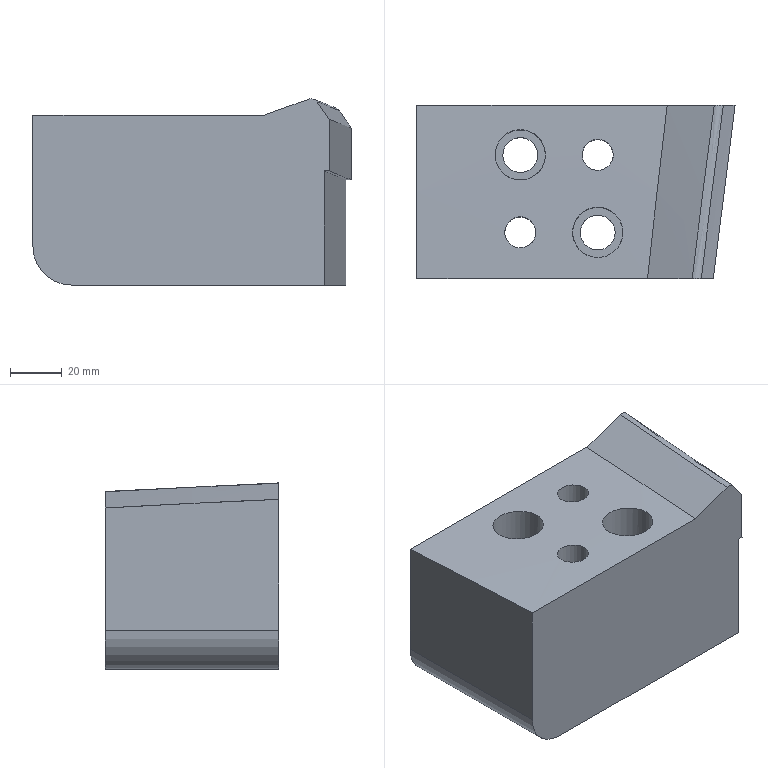Part | NX | features MAIN_BODY 2 | 1 solid | 20 faces | box 123.132 x 67 x 72.076 mm | volume 460289 mm3 | spline 7 | cylinder 7 | plane 6 | commonest cylinder face diameters 12 x2 13.5 x2 19.5 x2 30 x1
STEP:
#1=CARTESIAN_POINT('',(-841.75,399.358,-100.));
#2=VERTEX_POINT('',#1);
#3=CARTESIAN_POINT('',(-835.,399.358,-100.));
#4=DIRECTION('',(-0.000000341,-0.00000017,-1.));
#5=DIRECTION('',(-1.,0.,0.000000341));
#6=AXIS2_PLACEMENT_3D('',#3,#4,#5);
#7=CIRCLE('',#6,6.75);
#8=EDGE_CURVE('',#2,#2,#7,.F.);
#9=ORIENTED_EDGE('',*,*,#8,.T.);
#10=EDGE_LOOP('',(#9));
#11=FACE_BOUND('',#10,.T.);
#12=CARTESIAN_POINT('',(-841.,369.358,-100.));
#13=VERTEX_POINT('',#12);
#14=CARTESIAN_POINT('',(-835.,369.358,-100.));
#15=DIRECTION('',(-0.000000341,-0.00000017,-1.));
#16=DIRECTION('',(-1.,0.,0.000000341));
#17=AXIS2_PLACEMENT_3D('',#14,#15,#16);
#18=CIRCLE('',#17,6.);
#19=EDGE_CURVE('',#13,#13,#18,.F.);
#20=ORIENTED_EDGE('',*,*,#19,.T.);
#21=EDGE_LOOP('',(#20));
#22=FACE_BOUND('',#21,.T.);
#23=CARTESIAN_POINT('',(-811.75,369.358,-100.));
#24=VERTEX_POINT('',#23);
#25=CARTESIAN_POINT('',(-805.,369.358,-100.));
#26=DIRECTION('',(-0.000000341,-0.00000017,-1.));
#27=DIRECTION('',(-1.,0.,0.000000341));
#28=AXIS2_PLACEMENT_3D('',#25,#26,#27);
#29=CIRCLE('',#28,6.75);
#30=EDGE_CURVE('',#24,#24,#29,.F.);
#31=ORIENTED_EDGE('',*,*,#30,.T.);
#32=EDGE_LOOP('',(#31));
#33=FACE_BOUND('',#32,.T.);
#34=CARTESIAN_POINT('',(-811.,399.358,-100.));
#35=VERTEX_POINT('',#34);
#36=CARTESIAN_POINT('',(-805.,399.358,-100.));
#37=DIRECTION('',(-0.000000341,-0.00000017,-1.));
#38=DIRECTION('',(-1.,0.,0.000000341));
#39=AXIS2_PLACEMENT_3D('',#36,#37,#38);
#40=CIRCLE('',#39,6.);
#41=EDGE_CURVE('',#35,#35,#40,.F.);
#42=ORIENTED_EDGE('',*,*,#41,.T.);
#43=EDGE_LOOP('',(#42));
#44=FACE_BOUND('',#43,.T.);
#45=CARTESIAN_POINT('',(-860.,351.533,-100.));
#46=VERTEX_POINT('',#45);
#47=CARTESIAN_POINT('',(-762.297,351.533,-100.));
#48=VERTEX_POINT('',#47);
#49=CARTESIAN_POINT('',(-780.,351.533,-100.));
#50=DIRECTION('',(1.,0.000000011,-0.000000341));
#51=VECTOR('',#50,1000.);
#52=LINE('',#49,#51);
#53=EDGE_CURVE('',#46,#48,#52,.T.);
#54=ORIENTED_EDGE('',*,*,#53,.F.);
#55=CARTESIAN_POINT('',(-860.,418.533,-100.));
#56=VERTEX_POINT('',#55);
#57=CARTESIAN_POINT('',(-860.,1058.533,-100.));
#58=DIRECTION('',(-0.000000011,1.,-0.00000017));
#59=VECTOR('',#58,1000.);
#60=LINE('',#57,#59);
#61=EDGE_CURVE('',#46,#56,#60,.T.);
#62=ORIENTED_EDGE('',*,*,#61,.T.);
#63=CARTESIAN_POINT('',(-753.885,418.533,-100.));
#64=VERTEX_POINT('',#63);
#65=CARTESIAN_POINT('',(-780.,418.533,-100.));
#66=DIRECTION('',(1.,0.000000011,-0.000000341));
#67=VECTOR('',#66,1000.);
#68=LINE('',#65,#67);
#69=EDGE_CURVE('',#56,#64,#68,.T.);
#70=ORIENTED_EDGE('',*,*,#69,.T.);
#71=CARTESIAN_POINT('',(-753.885,418.533,-100.));
#72=CARTESIAN_POINT('',(-755.339,407.373,-100.));
#73=CARTESIAN_POINT('',(-758.303,385.059,-100.));
#74=CARTESIAN_POINT('',(-760.967,362.708,-100.));
#75=CARTESIAN_POINT('',(-762.297,351.533,-100.));
#76=B_SPLINE_CURVE_WITH_KNOTS('',3,(#71,#72,#73,#74,#75),.UNSPECIFIED.,.F.,.F.,(4,1,4),(0.2736,0.3074,0.3412),.UNSPECIFIED.);
#77=EDGE_CURVE('',#64,#48,#76,.T.);
#78=ORIENTED_EDGE('',*,*,#77,.T.);
#79=EDGE_LOOP('',(#54,#62,#70,#78));
#80=FACE_BOUND('',#79,.T.);
#81=CARTESIAN_POINT('',(-780.,1058.533,-100.));
#82=DIRECTION('',(-0.000000341,-0.00000017,-1.));
#83=DIRECTION('',(-0.000000011,1.,-0.00000017));
#84=AXIS2_PLACEMENT_3D('',#81,#82,#83);
#85=PLANE('',#84);
#86=ADVANCED_FACE('',(#11,#22,#33,#44,#80),#85,.T.);
#87=CARTESIAN_POINT('',(-751.868,418.533,-39.201));
#88=VERTEX_POINT('',#87);
#89=CARTESIAN_POINT('',(-756.435,418.533,-32.553));
#90=VERTEX_POINT('',#89);
#91=CARTESIAN_POINT('',(-751.868,418.533,-39.201));
#92=CARTESIAN_POINT('',(-753.39,418.533,-36.985));
#93=CARTESIAN_POINT('',(-754.912,418.533,-34.769));
#94=CARTESIAN_POINT('',(-756.435,418.533,-32.553));
#95=B_SPLINE_CURVE_WITH_KNOTS('',3,(#91,#92,#93,#94),.UNSPECIFIED.,.F.,.F.,(4,4),(0.,0.008065),.UNSPECIFIED.);
#96=EDGE_CURVE('',#88,#90,#95,.T.);
#97=ORIENTED_EDGE('',*,*,#96,.F.);
#98=CARTESIAN_POINT('',(-751.868,418.533,-59.201));
#99=VERTEX_POINT('',#98);
#100=CARTESIAN_POINT('',(-751.868,418.533,-39.201));
#101=CARTESIAN_POINT('',(-751.868,418.533,-45.868));
#102=CARTESIAN_POINT('',(-751.868,418.533,-52.535));
#103=CARTESIAN_POINT('',(-751.868,418.533,-59.201));
#104=B_SPLINE_CURVE_WITH_KNOTS('',3,(#100,#101,#102,#103),.UNSPECIFIED.,.F.,.F.,(4,4),(0.01625,0.03625),.UNSPECIFIED.);
#105=EDGE_CURVE('',#88,#99,#104,.T.);
#106=ORIENTED_EDGE('',*,*,#105,.T.);
#107=CARTESIAN_POINT('',(-753.885,418.533,-59.187));
#108=VERTEX_POINT('',#107);
#109=CARTESIAN_POINT('',(-753.885,418.533,-59.187));
#110=CARTESIAN_POINT('',(-753.213,418.533,-59.192));
#111=CARTESIAN_POINT('',(-752.541,418.533,-59.197));
#112=CARTESIAN_POINT('',(-751.868,418.533,-59.201));
#113=B_SPLINE_CURVE_WITH_KNOTS('',3,(#109,#110,#111,#112),.UNSPECIFIED.,.F.,.F.,(4,4),(0.,0.002017),.UNSPECIFIED.);
#114=EDGE_CURVE('',#108,#99,#113,.T.);
#115=ORIENTED_EDGE('',*,*,#114,.F.);
#116=CARTESIAN_POINT('',(-753.885,418.533,-59.187));
#117=CARTESIAN_POINT('',(-753.885,418.533,-72.791));
#118=CARTESIAN_POINT('',(-753.885,418.533,-86.396));
#119=CARTESIAN_POINT('',(-753.885,418.533,-100.));
#120=B_SPLINE_CURVE_WITH_KNOTS('',3,(#116,#117,#118,#119),.UNSPECIFIED.,.F.,.F.,(4,4),(-0.004527,0.03629),.UNSPECIFIED.);
#121=EDGE_CURVE('',#108,#64,#120,.T.);
#122=ORIENTED_EDGE('',*,*,#121,.T.);
#123=ORIENTED_EDGE('',*,*,#69,.F.);
#124=CARTESIAN_POINT('',(-875.,418.533,-85.));
#125=VERTEX_POINT('',#124);
#126=CARTESIAN_POINT('',(-860.,418.533,-85.));
#127=DIRECTION('',(-0.000000011,1.,-0.00000017));
#128=DIRECTION('',(0.,0.00000017,1.));
#129=AXIS2_PLACEMENT_3D('',#126,#127,#128);
#130=CIRCLE('',#129,15.);
#131=EDGE_CURVE('',#56,#125,#130,.T.);
#132=ORIENTED_EDGE('',*,*,#131,.T.);
#133=CARTESIAN_POINT('',(-875.,418.533,-37.652));
#134=VERTEX_POINT('',#133);
#135=CARTESIAN_POINT('',(-875.,418.533,-90.));
#136=DIRECTION('',(-0.000000341,-0.00000017,-1.));
#137=VECTOR('',#136,1000.);
#138=LINE('',#135,#137);
#139=EDGE_CURVE('',#125,#134,#138,.F.);
#140=ORIENTED_EDGE('',*,*,#139,.T.);
#141=CARTESIAN_POINT('',(-778.148,418.533,-37.652));
#142=VERTEX_POINT('',#141);
#143=CARTESIAN_POINT('',(-820.117,418.533,-37.652));
#144=DIRECTION('',(1.,0.000000011,-0.000000341));
#145=VECTOR('',#144,1000.);
#146=LINE('',#143,#145);
#147=EDGE_CURVE('',#134,#142,#146,.T.);
#148=ORIENTED_EDGE('',*,*,#147,.T.);
#149=CARTESIAN_POINT('',(-759.941,418.533,-31.393));
#150=VERTEX_POINT('',#149);
#151=CARTESIAN_POINT('',(-759.941,418.533,-31.393));
#152=CARTESIAN_POINT('',(-766.01,418.533,-33.479));
#153=CARTESIAN_POINT('',(-772.079,418.533,-35.565));
#154=CARTESIAN_POINT('',(-778.148,418.533,-37.652));
#155=B_SPLINE_CURVE_WITH_KNOTS('',3,(#151,#152,#153,#154),.UNSPECIFIED.,.F.,.F.,(4,4),(0.02556,0.04482),.UNSPECIFIED.);
#156=EDGE_CURVE('',#150,#142,#155,.T.);
#157=ORIENTED_EDGE('',*,*,#156,.F.);
#158=CARTESIAN_POINT('',(-756.435,418.533,-32.553));
#159=CARTESIAN_POINT('',(-757.19,418.533,-31.454));
#160=CARTESIAN_POINT('',(-758.679,418.533,-30.959));
#161=CARTESIAN_POINT('',(-759.941,418.533,-31.393));
#162=B_SPLINE_CURVE_WITH_KNOTS('',3,(#158,#159,#160,#161),.UNSPECIFIED.,.F.,.F.,(4,4),(0.,0.003944),.UNSPECIFIED.);
#163=EDGE_CURVE('',#90,#150,#162,.T.);
#164=ORIENTED_EDGE('',*,*,#163,.F.);
#165=EDGE_LOOP('',(#97,#106,#115,#122,#123,#132,#140,#148,#157,#164));
#166=FACE_BOUND('',#165,.T.);
#167=CARTESIAN_POINT('',(-840.,418.533,-90.));
#168=DIRECTION('',(-0.000000011,1.,-0.00000017));
#169=DIRECTION('',(0.000000341,0.00000017,1.));
#170=AXIS2_PLACEMENT_3D('',#167,#168,#169);
#171=PLANE('',#170);
#172=ADVANCED_FACE('',(#166),#171,.T.);
#173=CARTESIAN_POINT('',(-760.283,351.533,-35.819));
#174=VERTEX_POINT('',#173);
#175=CARTESIAN_POINT('',(-760.283,351.533,-55.819));
#176=VERTEX_POINT('',#175);
#177=CARTESIAN_POINT('',(-760.283,351.533,-35.819));
#178=CARTESIAN_POINT('',(-760.283,351.533,-42.486));
#179=CARTESIAN_POINT('',(-760.283,351.533,-49.152));
#180=CARTESIAN_POINT('',(-760.283,351.533,-55.819));
#181=B_SPLINE_CURVE_WITH_KNOTS('',3,(#177,#178,#179,#180),.UNSPECIFIED.,.F.,.F.,(4,4),(0.009058,0.02906),.UNSPECIFIED.);
#182=EDGE_CURVE('',#174,#176,#181,.T.);
#183=ORIENTED_EDGE('',*,*,#182,.T.);
#184=CARTESIAN_POINT('',(-751.868,418.533,-59.201));
#185=CARTESIAN_POINT('',(-753.322,407.375,-58.596));
#186=CARTESIAN_POINT('',(-756.286,385.067,-57.354));
#187=CARTESIAN_POINT('',(-758.953,362.711,-56.325));
#188=CARTESIAN_POINT('',(-760.283,351.533,-55.819));
#189=B_SPLINE_CURVE_WITH_KNOTS('',3,(#184,#185,#186,#187,#188),.UNSPECIFIED.,.F.,.F.,(4,1,4),(0.,0.03381,0.06761),.UNSPECIFIED.);
#190=EDGE_CURVE('',#99,#176,#189,.T.);
#191=ORIENTED_EDGE('',*,*,#190,.F.);
#192=ORIENTED_EDGE('',*,*,#105,.F.);
#193=CARTESIAN_POINT('',(-760.283,351.533,-35.819));
#194=CARTESIAN_POINT('',(-758.953,362.711,-36.325));
#195=CARTESIAN_POINT('',(-756.286,385.067,-37.354));
#196=CARTESIAN_POINT('',(-753.322,407.375,-38.596));
#197=CARTESIAN_POINT('',(-751.868,418.533,-39.201));
#198=B_SPLINE_CURVE_WITH_KNOTS('',3,(#193,#194,#195,#196,#197),.UNSPECIFIED.,.F.,.F.,(4,1,4),(0.,0.03381,0.06761),.UNSPECIFIED.);
#199=EDGE_CURVE('',#174,#88,#198,.T.);
#200=ORIENTED_EDGE('',*,*,#199,.F.);
#201=EDGE_LOOP('',(#183,#191,#192,#200));
#202=FACE_BOUND('',#201,.T.);
#203=CARTESIAN_POINT('',(-760.331,351.13,-55.941));
#204=CARTESIAN_POINT('',(-760.331,351.13,-35.657));
#205=CARTESIAN_POINT('',(-758.993,362.375,-56.467));
#206=CARTESIAN_POINT('',(-758.993,362.375,-36.183));
#207=CARTESIAN_POINT('',(-756.313,384.864,-57.522));
#208=CARTESIAN_POINT('',(-756.313,384.864,-37.238));
#209=CARTESIAN_POINT('',(-753.331,407.307,-58.731));
#210=CARTESIAN_POINT('',(-753.331,407.307,-38.447));
#211=CARTESIAN_POINT('',(-751.868,418.533,-59.322));
#212=CARTESIAN_POINT('',(-751.868,418.533,-39.037));
#213=B_SPLINE_SURFACE_WITH_KNOTS('',3,1,((#203,#204),(#205,#206),(#207,#208),(#209,#210),(#211,#212)),.SURF_OF_LINEAR_EXTRUSION.,.F.,.F.,.F.,(4,1,4),(2,2),(-0.3914,0.6746,1.741),(0.,1.),.UNSPECIFIED.);
#214=ADVANCED_FACE('',(#202),#213,.T.);
#215=ORIENTED_EDGE('',*,*,#139,.F.);
#216=CARTESIAN_POINT('',(-875.,351.533,-85.));
#217=VERTEX_POINT('',#216);
#218=CARTESIAN_POINT('',(-875.,739.25,-85.));
#219=DIRECTION('',(0.000000011,-1.,0.00000017));
#220=VECTOR('',#219,1000.);
#221=LINE('',#218,#220);
#222=EDGE_CURVE('',#125,#217,#221,.T.);
#223=ORIENTED_EDGE('',*,*,#222,.T.);
#224=CARTESIAN_POINT('',(-875.,351.533,-34.317));
#225=VERTEX_POINT('',#224);
#226=CARTESIAN_POINT('',(-875.,351.533,-90.));
#227=DIRECTION('',(-0.000000341,-0.00000017,-1.));
#228=VECTOR('',#227,1000.);
#229=LINE('',#226,#228);
#230=EDGE_CURVE('',#217,#225,#229,.F.);
#231=ORIENTED_EDGE('',*,*,#230,.T.);
#232=CARTESIAN_POINT('',(-875.,351.533,-34.317));
#233=CARTESIAN_POINT('',(-875.,373.874,-35.265));
#234=CARTESIAN_POINT('',(-875.,396.208,-36.367));
#235=CARTESIAN_POINT('',(-875.,418.533,-37.652));
#236=B_SPLINE_CURVE_WITH_KNOTS('',3,(#232,#233,#234,#235),.UNSPECIFIED.,.F.,.F.,(4,4),(0.277,0.3441),.UNSPECIFIED.);
#237=EDGE_CURVE('',#134,#225,#236,.F.);
#238=ORIENTED_EDGE('',*,*,#237,.F.);
#239=EDGE_LOOP('',(#215,#223,#231,#238));
#240=FACE_BOUND('',#239,.T.);
#241=CARTESIAN_POINT('',(-875.,739.25,-90.));
#242=DIRECTION('',(-1.,-0.000000011,0.000000341));
#243=DIRECTION('',(-0.000000341,-0.00000017,-1.));
#244=AXIS2_PLACEMENT_3D('',#241,#242,#243);
#245=PLANE('',#244);
#246=ADVANCED_FACE('',(#240),#245,.T.);
#247=CARTESIAN_POINT('',(-802.615,378.812,-35.56));
#248=VERTEX_POINT('',#247);
#249=CARTESIAN_POINT('',(-810.554,378.63,-35.551));
#250=CARTESIAN_POINT('',(-802.353,379.838,-35.61));
#251=CARTESIAN_POINT('',(-795.722,374.891,-35.371));
#252=CARTESIAN_POINT('',(-794.523,366.727,-34.987));
#253=CARTESIAN_POINT('',(-799.45,360.085,-34.688));
#254=CARTESIAN_POINT('',(-807.643,358.881,-34.635));
#255=CARTESIAN_POINT('',(-814.27,363.813,-34.854));
#256=CARTESIAN_POINT('',(-815.479,371.987,-35.232));
#257=CARTESIAN_POINT('',(-810.554,378.63,-35.551));
#258=CARTESIAN_POINT('',(-802.353,379.838,-35.61));
#259=CARTESIAN_POINT('',(-795.722,374.891,-35.371));
#260=B_SPLINE_CURVE_WITH_KNOTS('',3,(#249,#250,#251,#252,#253,#254,#255,#256,#257,#258,#259),.UNSPECIFIED.,.T.,.F.,(1,1,1,1,1,1,1,1,1,1,1,1,1,1,1),(-0.02287,-0.01525,-0.007624,0.,0.007624,0.01525,0.02287,0.0305,0.03812,0.04574,0.05337,0.06099,0.06862,0.07624,0.08386),.UNSPECIFIED.);
#261=EDGE_CURVE('',#248,#248,#260,.T.);
#262=ORIENTED_EDGE('',*,*,#261,.T.);
#263=EDGE_LOOP('',(#262));
#264=FACE_BOUND('',#263,.T.);
#265=CARTESIAN_POINT('',(-806.104,405.256,-36.91));
#266=VERTEX_POINT('',#265);
#267=CARTESIAN_POINT('',(-810.492,403.108,-36.793));
#268=CARTESIAN_POINT('',(-806.223,405.897,-36.944));
#269=CARTESIAN_POINT('',(-801.239,404.841,-36.887));
#270=CARTESIAN_POINT('',(-798.467,400.584,-36.658));
#271=CARTESIAN_POINT('',(-799.51,395.607,-36.398));
#272=CARTESIAN_POINT('',(-803.775,392.823,-36.256));
#273=CARTESIAN_POINT('',(-808.753,393.871,-36.309));
#274=CARTESIAN_POINT('',(-811.534,398.131,-36.529));
#275=CARTESIAN_POINT('',(-810.492,403.108,-36.793));
#276=CARTESIAN_POINT('',(-806.223,405.897,-36.944));
#277=CARTESIAN_POINT('',(-801.239,404.841,-36.887));
#278=B_SPLINE_CURVE_WITH_KNOTS('',3,(#267,#268,#269,#270,#271,#272,#273,#274,#275,#276,#277),.UNSPECIFIED.,.T.,.F.,(1,1,1,1,1,1,1,1,1,1,1,1,1,1,1),(-0.01408,-0.009385,-0.004692,0.,0.004692,0.009385,0.01408,0.01877,0.02346,0.02815,0.03285,0.03754,0.04223,0.04692,0.05162),.UNSPECIFIED.);
#279=EDGE_CURVE('',#266,#266,#278,.T.);
#280=ORIENTED_EDGE('',*,*,#279,.T.);
#281=EDGE_LOOP('',(#280));
#282=FACE_BOUND('',#281,.T.);
#283=CARTESIAN_POINT('',(-785.768,351.533,-34.317));
#284=VERTEX_POINT('',#283);
#285=CARTESIAN_POINT('',(-823.992,351.533,-34.317));
#286=DIRECTION('',(1.,0.000000011,-0.000000341));
#287=VECTOR('',#286,1000.);
#288=LINE('',#285,#287);
#289=EDGE_CURVE('',#225,#284,#288,.T.);
#290=ORIENTED_EDGE('',*,*,#289,.T.);
#291=CARTESIAN_POINT('',(-778.148,418.533,-37.652));
#292=CARTESIAN_POINT('',(-780.817,396.223,-36.368));
#293=CARTESIAN_POINT('',(-783.364,373.889,-35.266));
#294=CARTESIAN_POINT('',(-785.768,351.533,-34.317));
#295=B_SPLINE_CURVE_WITH_KNOTS('',3,(#291,#292,#293,#294),.UNSPECIFIED.,.F.,.F.,(4,4),(0.1671,0.2344),.UNSPECIFIED.);
#296=EDGE_CURVE('',#142,#284,#295,.T.);
#297=ORIENTED_EDGE('',*,*,#296,.F.);
#298=ORIENTED_EDGE('',*,*,#147,.F.);
#299=ORIENTED_EDGE('',*,*,#237,.T.);
#300=EDGE_LOOP('',(#290,#297,#298,#299));
#301=FACE_BOUND('',#300,.T.);
#302=CARTESIAN_POINT('',(-837.117,374.973,-35.376));
#303=VERTEX_POINT('',#302);
#304=CARTESIAN_POINT('',(-841.061,372.092,-35.239));
#305=CARTESIAN_POINT('',(-837.346,375.582,-35.405));
#306=CARTESIAN_POINT('',(-832.255,375.414,-35.397));
#307=CARTESIAN_POINT('',(-828.781,371.706,-35.22));
#308=CARTESIAN_POINT('',(-828.94,366.622,-34.983));
#309=CARTESIAN_POINT('',(-832.652,363.137,-34.825));
#310=CARTESIAN_POINT('',(-837.736,363.299,-34.832));
#311=CARTESIAN_POINT('',(-841.22,367.009,-35.001));
#312=CARTESIAN_POINT('',(-841.061,372.092,-35.239));
#313=CARTESIAN_POINT('',(-837.346,375.582,-35.405));
#314=CARTESIAN_POINT('',(-832.255,375.414,-35.397));
#315=B_SPLINE_CURVE_WITH_KNOTS('',3,(#304,#305,#306,#307,#308,#309,#310,#311,#312,#313,#314),.UNSPECIFIED.,.T.,.F.,(1,1,1,1,1,1,1,1,1,1,1,1,1,1,1),(-0.01408,-0.009384,-0.004692,0.,0.004692,0.009384,0.01408,0.01877,0.02346,0.02815,0.03284,0.03753,0.04223,0.04692,0.05161),.UNSPECIFIED.);
#316=EDGE_CURVE('',#303,#303,#315,.T.);
#317=ORIENTED_EDGE('',*,*,#316,.T.);
#318=EDGE_LOOP('',(#317));
#319=FACE_BOUND('',#318,.T.);
#320=CARTESIAN_POINT('',(-844.701,400.333,-36.646));
#321=VERTEX_POINT('',#320);
#322=CARTESIAN_POINT('',(-843.364,392.516,-36.238));
#323=CARTESIAN_POINT('',(-845.751,400.44,-36.648));
#324=CARTESIAN_POINT('',(-841.839,407.721,-37.043));
#325=CARTESIAN_POINT('',(-833.927,410.11,-37.176));
#326=CARTESIAN_POINT('',(-826.634,406.198,-36.959));
#327=CARTESIAN_POINT('',(-824.252,398.282,-36.535));
#328=CARTESIAN_POINT('',(-828.148,391.005,-36.162));
#329=CARTESIAN_POINT('',(-836.069,388.604,-36.043));
#330=CARTESIAN_POINT('',(-843.364,392.516,-36.238));
#331=CARTESIAN_POINT('',(-845.751,400.44,-36.648));
#332=CARTESIAN_POINT('',(-841.839,407.721,-37.043));
#333=B_SPLINE_CURVE_WITH_KNOTS('',3,(#322,#323,#324,#325,#326,#327,#328,#329,#330,#331,#332),.UNSPECIFIED.,.T.,.F.,(1,1,1,1,1,1,1,1,1,1,1,1,1,1,1),(-0.02288,-0.01525,-0.007625,0.,0.007625,0.01525,0.02288,0.0305,0.03813,0.04575,0.05338,0.061,0.06863,0.07625,0.08388),.UNSPECIFIED.);
#334=EDGE_CURVE('',#321,#321,#333,.T.);
#335=ORIENTED_EDGE('',*,*,#334,.T.);
#336=EDGE_LOOP('',(#335));
#337=FACE_BOUND('',#336,.T.);
#338=CARTESIAN_POINT('',(-875.586,418.533,-37.652));
#339=CARTESIAN_POINT('',(-776.779,418.533,-37.652));
#340=CARTESIAN_POINT('',(-877.041,407.36,-37.009));
#341=CARTESIAN_POINT('',(-778.234,407.36,-37.009));
#342=CARTESIAN_POINT('',(-880.005,385.084,-35.832));
#343=CARTESIAN_POINT('',(-781.198,385.084,-35.832));
#344=CARTESIAN_POINT('',(-882.657,362.711,-34.791));
#345=CARTESIAN_POINT('',(-783.85,362.711,-34.791));
#346=CARTESIAN_POINT('',(-883.99,351.533,-34.317));
#347=CARTESIAN_POINT('',(-785.183,351.533,-34.317));
#348=B_SPLINE_SURFACE_WITH_KNOTS('',3,1,((#338,#339),(#340,#341),(#342,#343),(#344,#345),(#346,#347)),.SURF_OF_LINEAR_EXTRUSION.,.F.,.F.,.F.,(4,1,4),(2,2),(-0.00601,0.4948,0.9956),(0.,1.),.UNSPECIFIED.);
#349=ADVANCED_FACE('',(#264,#282,#301,#319,#337),#348,.T.);
#350=CARTESIAN_POINT('',(-768.455,351.533,-28.093));
#351=VERTEX_POINT('',#350);
#352=CARTESIAN_POINT('',(-785.768,351.533,-34.317));
#353=CARTESIAN_POINT('',(-779.997,351.533,-32.242));
#354=CARTESIAN_POINT('',(-774.226,351.533,-30.167));
#355=CARTESIAN_POINT('',(-768.455,351.533,-28.093));
#356=B_SPLINE_CURVE_WITH_KNOTS('',3,(#352,#353,#354,#355),.UNSPECIFIED.,.F.,.F.,(4,4),(0.07252,0.09092),.UNSPECIFIED.);
#357=EDGE_CURVE('',#351,#284,#356,.F.);
#358=ORIENTED_EDGE('',*,*,#357,.T.);
#359=ORIENTED_EDGE('',*,*,#289,.F.);
#360=ORIENTED_EDGE('',*,*,#230,.F.);
#361=CARTESIAN_POINT('',(-860.,351.533,-85.));
#362=DIRECTION('',(-0.000000011,1.,-0.00000017));
#363=DIRECTION('',(0.,0.00000017,1.));
#364=AXIS2_PLACEMENT_3D('',#361,#362,#363);
#365=CIRCLE('',#364,15.);
#366=EDGE_CURVE('',#217,#46,#365,.F.);
#367=ORIENTED_EDGE('',*,*,#366,.T.);
#368=ORIENTED_EDGE('',*,*,#53,.T.);
#369=CARTESIAN_POINT('',(-762.297,351.533,-55.808));
#370=VERTEX_POINT('',#369);
#371=CARTESIAN_POINT('',(-762.297,351.533,-55.808));
#372=CARTESIAN_POINT('',(-762.297,351.533,-70.539));
#373=CARTESIAN_POINT('',(-762.297,351.533,-85.269));
#374=CARTESIAN_POINT('',(-762.297,351.533,-100.));
#375=B_SPLINE_CURVE_WITH_KNOTS('',3,(#371,#372,#373,#374),.UNSPECIFIED.,.F.,.F.,(4,4),(-0.01041,0.03379),.UNSPECIFIED.);
#376=EDGE_CURVE('',#370,#48,#375,.T.);
#377=ORIENTED_EDGE('',*,*,#376,.F.);
#378=CARTESIAN_POINT('',(-760.283,351.533,-55.819));
#379=CARTESIAN_POINT('',(-760.955,351.533,-55.816));
#380=CARTESIAN_POINT('',(-761.626,351.533,-55.812));
#381=CARTESIAN_POINT('',(-762.297,351.533,-55.808));
#382=B_SPLINE_CURVE_WITH_KNOTS('',3,(#378,#379,#380,#381),.UNSPECIFIED.,.F.,.F.,(4,4),(0.,0.002014),.UNSPECIFIED.);
#383=EDGE_CURVE('',#176,#370,#382,.T.);
#384=ORIENTED_EDGE('',*,*,#383,.F.);
#385=ORIENTED_EDGE('',*,*,#182,.F.);
#386=CARTESIAN_POINT('',(-764.943,351.533,-29.203));
#387=VERTEX_POINT('',#386);
#388=CARTESIAN_POINT('',(-764.943,351.533,-29.203));
#389=CARTESIAN_POINT('',(-763.39,351.533,-31.408));
#390=CARTESIAN_POINT('',(-761.836,351.533,-33.614));
#391=CARTESIAN_POINT('',(-760.283,351.533,-35.819));
#392=B_SPLINE_CURVE_WITH_KNOTS('',3,(#388,#389,#390,#391),.UNSPECIFIED.,.F.,.F.,(4,4),(0.007518,0.01561),.UNSPECIFIED.);
#393=EDGE_CURVE('',#387,#174,#392,.T.);
#394=ORIENTED_EDGE('',*,*,#393,.F.);
#395=CARTESIAN_POINT('',(-768.455,351.533,-28.093));
#396=CARTESIAN_POINT('',(-767.203,351.533,-27.643));
#397=CARTESIAN_POINT('',(-765.71,351.533,-28.115));
#398=CARTESIAN_POINT('',(-764.943,351.533,-29.203));
#399=B_SPLINE_CURVE_WITH_KNOTS('',3,(#395,#396,#397,#398),.UNSPECIFIED.,.F.,.F.,(4,4),(0.,0.003935),.UNSPECIFIED.);
#400=EDGE_CURVE('',#351,#387,#399,.T.);
#401=ORIENTED_EDGE('',*,*,#400,.F.);
#402=EDGE_LOOP('',(#358,#359,#360,#367,#368,#377,#384,#385,#394,#401));
#403=FACE_BOUND('',#402,.T.);
#404=CARTESIAN_POINT('',(-840.,351.533,-90.));
#405=DIRECTION('',(-0.000000011,1.,-0.00000017));
#406=DIRECTION('',(0.000000341,0.00000017,1.));
#407=AXIS2_PLACEMENT_3D('',#404,#405,#406);
#408=PLANE('',#407);
#409=ADVANCED_FACE('',(#403),#408,.F.);
#410=CARTESIAN_POINT('',(-844.75,399.358,-80.));
#411=VERTEX_POINT('',#410);
#412=CARTESIAN_POINT('',(-835.,399.358,-80.));
#413=DIRECTION('',(-0.000000341,-0.00000017,-1.));
#414=DIRECTION('',(-1.,0.,0.000000341));
#415=AXIS2_PLACEMENT_3D('',#412,#413,#414);
#416=CIRCLE('',#415,9.75);
#417=EDGE_CURVE('',#411,#411,#416,.F.);
#418=ORIENTED_EDGE('',*,*,#417,.F.);
#419=EDGE_LOOP('',(#418));
#420=FACE_BOUND('',#419,.T.);
#421=ORIENTED_EDGE('',*,*,#334,.F.);
#422=EDGE_LOOP('',(#421));
#423=FACE_BOUND('',#422,.T.);
#424=CARTESIAN_POINT('',(-835.,399.358,-70.));
#425=DIRECTION('',(0.000000341,0.00000017,1.));
#426=DIRECTION('',(0.000000011,-1.,0.00000017));
#427=AXIS2_PLACEMENT_3D('',#424,#425,#426);
#428=CYLINDRICAL_SURFACE('',#427,9.75);
#429=ADVANCED_FACE('',(#420,#423),#428,.F.);
#430=CARTESIAN_POINT('',(-841.75,399.358,-80.));
#431=VERTEX_POINT('',#430);
#432=CARTESIAN_POINT('',(-835.,399.358,-80.));
#433=DIRECTION('',(-0.000000341,-0.00000017,-1.));
#434=DIRECTION('',(-1.,0.,0.000000341));
#435=AXIS2_PLACEMENT_3D('',#432,#433,#434);
#436=CIRCLE('',#435,6.75);
#437=EDGE_CURVE('',#431,#431,#436,.F.);
#438=ORIENTED_EDGE('',*,*,#437,.T.);
#439=EDGE_LOOP('',(#438));
#440=FACE_BOUND('',#439,.T.);
#441=ORIENTED_EDGE('',*,*,#8,.F.);
#442=EDGE_LOOP('',(#441));
#443=FACE_BOUND('',#442,.T.);
#444=CARTESIAN_POINT('',(-835.,399.358,-90.));
#445=DIRECTION('',(0.000000341,0.00000017,1.));
#446=DIRECTION('',(0.000000011,-1.,0.00000017));
#447=AXIS2_PLACEMENT_3D('',#444,#445,#446);
#448=CYLINDRICAL_SURFACE('',#447,6.75);
#449=ADVANCED_FACE('',(#440,#443),#448,.F.);
#450=ORIENTED_EDGE('',*,*,#437,.F.);
#451=EDGE_LOOP('',(#450));
#452=FACE_BOUND('',#451,.T.);
#453=ORIENTED_EDGE('',*,*,#417,.T.);
#454=EDGE_LOOP('',(#453));
#455=FACE_BOUND('',#454,.T.);
#456=CARTESIAN_POINT('',(-835.,399.358,-80.));
#457=DIRECTION('',(-0.000000341,-0.00000017,-1.));
#458=DIRECTION('',(-0.000000011,1.,-0.00000017));
#459=AXIS2_PLACEMENT_3D('',#456,#457,#458);
#460=PLANE('',#459);
#461=ADVANCED_FACE('',(#452,#455),#460,.F.);
#462=ORIENTED_EDGE('',*,*,#19,.F.);
#463=EDGE_LOOP('',(#462));
#464=FACE_BOUND('',#463,.T.);
#465=ORIENTED_EDGE('',*,*,#316,.F.);
#466=EDGE_LOOP('',(#465));
#467=FACE_BOUND('',#466,.T.);
#468=CARTESIAN_POINT('',(-835.,369.358,-90.));
#469=DIRECTION('',(0.000000341,0.00000017,1.));
#470=DIRECTION('',(0.000000011,-1.,0.00000017));
#471=AXIS2_PLACEMENT_3D('',#468,#469,#470);
#472=CYLINDRICAL_SURFACE('',#471,6.);
#473=ADVANCED_FACE('',(#464,#467),#472,.F.);
#474=CARTESIAN_POINT('',(-814.75,369.358,-80.));
#475=VERTEX_POINT('',#474);
#476=CARTESIAN_POINT('',(-805.,369.358,-80.));
#477=DIRECTION('',(-0.000000341,-0.00000017,-1.));
#478=DIRECTION('',(-1.,0.,0.000000341));
#479=AXIS2_PLACEMENT_3D('',#476,#477,#478);
#480=CIRCLE('',#479,9.75);
#481=EDGE_CURVE('',#475,#475,#480,.F.);
#482=ORIENTED_EDGE('',*,*,#481,.F.);
#483=EDGE_LOOP('',(#482));
#484=FACE_BOUND('',#483,.T.);
#485=ORIENTED_EDGE('',*,*,#261,.F.);
#486=EDGE_LOOP('',(#485));
#487=FACE_BOUND('',#486,.T.);
#488=CARTESIAN_POINT('',(-805.,369.358,-70.));
#489=DIRECTION('',(0.000000341,0.00000017,1.));
#490=DIRECTION('',(0.000000011,-1.,0.00000017));
#491=AXIS2_PLACEMENT_3D('',#488,#489,#490);
#492=CYLINDRICAL_SURFACE('',#491,9.75);
#493=ADVANCED_FACE('',(#484,#487),#492,.F.);
#494=CARTESIAN_POINT('',(-811.75,369.358,-80.));
#495=VERTEX_POINT('',#494);
#496=CARTESIAN_POINT('',(-805.,369.358,-80.));
#497=DIRECTION('',(-0.000000341,-0.00000017,-1.));
#498=DIRECTION('',(-1.,0.,0.000000341));
#499=AXIS2_PLACEMENT_3D('',#496,#497,#498);
#500=CIRCLE('',#499,6.75);
#501=EDGE_CURVE('',#495,#495,#500,.F.);
#502=ORIENTED_EDGE('',*,*,#501,.T.);
#503=EDGE_LOOP('',(#502));
#504=FACE_BOUND('',#503,.T.);
#505=ORIENTED_EDGE('',*,*,#30,.F.);
#506=EDGE_LOOP('',(#505));
#507=FACE_BOUND('',#506,.T.);
#508=CARTESIAN_POINT('',(-805.,369.358,-90.));
#509=DIRECTION('',(0.000000341,0.00000017,1.));
#510=DIRECTION('',(0.000000011,-1.,0.00000017));
#511=AXIS2_PLACEMENT_3D('',#508,#509,#510);
#512=CYLINDRICAL_SURFACE('',#511,6.75);
#513=ADVANCED_FACE('',(#504,#507),#512,.F.);
#514=ORIENTED_EDGE('',*,*,#501,.F.);
#515=EDGE_LOOP('',(#514));
#516=FACE_BOUND('',#515,.T.);
#517=ORIENTED_EDGE('',*,*,#481,.T.);
#518=EDGE_LOOP('',(#517));
#519=FACE_BOUND('',#518,.T.);
#520=CARTESIAN_POINT('',(-805.,369.358,-80.));
#521=DIRECTION('',(-0.000000341,-0.00000017,-1.));
#522=DIRECTION('',(-0.000000011,1.,-0.00000017));
#523=AXIS2_PLACEMENT_3D('',#520,#521,#522);
#524=PLANE('',#523);
#525=ADVANCED_FACE('',(#516,#519),#524,.F.);
#526=ORIENTED_EDGE('',*,*,#41,.F.);
#527=EDGE_LOOP('',(#526));
#528=FACE_BOUND('',#527,.T.);
#529=ORIENTED_EDGE('',*,*,#279,.F.);
#530=EDGE_LOOP('',(#529));
#531=FACE_BOUND('',#530,.T.);
#532=CARTESIAN_POINT('',(-805.,399.358,-90.));
#533=DIRECTION('',(0.000000341,0.00000017,1.));
#534=DIRECTION('',(0.000000011,-1.,0.00000017));
#535=AXIS2_PLACEMENT_3D('',#532,#533,#534);
#536=CYLINDRICAL_SURFACE('',#535,6.);
#537=ADVANCED_FACE('',(#528,#531),#536,.F.);
#538=ORIENTED_EDGE('',*,*,#114,.T.);
#539=ORIENTED_EDGE('',*,*,#190,.T.);
#540=ORIENTED_EDGE('',*,*,#383,.T.);
#541=CARTESIAN_POINT('',(-753.885,418.533,-59.187));
#542=CARTESIAN_POINT('',(-755.339,407.375,-58.581));
#543=CARTESIAN_POINT('',(-758.302,385.067,-57.341));
#544=CARTESIAN_POINT('',(-760.967,362.711,-56.314));
#545=CARTESIAN_POINT('',(-762.297,351.533,-55.808));
#546=B_SPLINE_CURVE_WITH_KNOTS('',3,(#541,#542,#543,#544,#545),.UNSPECIFIED.,.F.,.F.,(4,1,4),(0.,0.03381,0.06761),.UNSPECIFIED.);
#547=EDGE_CURVE('',#108,#370,#546,.T.);
#548=ORIENTED_EDGE('',*,*,#547,.F.);
#549=EDGE_LOOP('',(#538,#539,#540,#548));
#550=FACE_BOUND('',#549,.T.);
#551=CARTESIAN_POINT('',(-751.849,418.53,-59.201));
#552=CARTESIAN_POINT('',(-753.303,407.372,-58.596));
#553=CARTESIAN_POINT('',(-754.778,396.218,-57.973));
#554=CARTESIAN_POINT('',(-757.606,373.887,-56.841));
#555=CARTESIAN_POINT('',(-758.933,362.709,-56.325));
#556=CARTESIAN_POINT('',(-760.264,351.53,-55.819));
#557=CARTESIAN_POINT('',(-760.289,351.317,-55.809));
#558=CARTESIAN_POINT('',(-760.314,351.104,-55.8));
#559=CARTESIAN_POINT('',(-760.34,350.89,-55.79));
#560=CARTESIAN_POINT('',(-753.869,418.793,-59.201));
#561=CARTESIAN_POINT('',(-755.323,407.637,-58.596));
#562=CARTESIAN_POINT('',(-756.799,396.482,-57.973));
#563=CARTESIAN_POINT('',(-759.629,374.135,-56.841));
#564=CARTESIAN_POINT('',(-760.957,362.946,-56.325));
#565=CARTESIAN_POINT('',(-762.287,351.771,-55.819));
#566=CARTESIAN_POINT('',(-762.312,351.558,-55.809));
#567=CARTESIAN_POINT('',(-762.338,351.344,-55.8));
#568=CARTESIAN_POINT('',(-762.363,351.131,-55.79));
#569=B_SPLINE_SURFACE_WITH_KNOTS('',1,3,((#551,#552,#553,#554,#555,#556,#557,#558,#559),(#560,#561,#562,#563,#564,#565,#566,#567,#568)),.RULED_SURF.,.F.,.F.,.F.,(2,2),(4,2,3,4),(0.498,0.7018),(0.,0.5,1.,1.01),.UNSPECIFIED.);
#570=ADVANCED_FACE('',(#550),#569,.F.);
#571=ORIENTED_EDGE('',*,*,#547,.T.);
#572=ORIENTED_EDGE('',*,*,#376,.T.);
#573=ORIENTED_EDGE('',*,*,#77,.F.);
#574=ORIENTED_EDGE('',*,*,#121,.F.);
#575=EDGE_LOOP('',(#571,#572,#573,#574));
#576=FACE_BOUND('',#575,.T.);
#577=CARTESIAN_POINT('',(-762.345,351.13,-100.246));
#578=CARTESIAN_POINT('',(-762.345,351.13,-55.499));
#579=CARTESIAN_POINT('',(-760.999,362.438,-100.776));
#580=CARTESIAN_POINT('',(-760.999,362.438,-56.029));
#581=CARTESIAN_POINT('',(-758.303,385.072,-101.836));
#582=CARTESIAN_POINT('',(-758.303,385.072,-57.089));
#583=CARTESIAN_POINT('',(-755.304,407.645,-103.052));
#584=CARTESIAN_POINT('',(-755.304,407.645,-58.305));
#585=CARTESIAN_POINT('',(-753.833,418.934,-103.646));
#586=CARTESIAN_POINT('',(-753.833,418.934,-58.899));
#587=B_SPLINE_SURFACE_WITH_KNOTS('',3,1,((#577,#578),(#579,#580),(#581,#582),(#583,#584),(#585,#586)),.SURF_OF_LINEAR_EXTRUSION.,.F.,.F.,.F.,(4,1,4),(2,2),(-0.3989,0.6732,1.745),(0.,1.),.UNSPECIFIED.);
#588=ADVANCED_FACE('',(#576),#587,.T.);
#589=ORIENTED_EDGE('',*,*,#131,.F.);
#590=ORIENTED_EDGE('',*,*,#61,.F.);
#591=ORIENTED_EDGE('',*,*,#366,.F.);
#592=ORIENTED_EDGE('',*,*,#222,.F.);
#593=EDGE_LOOP('',(#589,#590,#591,#592));
#594=FACE_BOUND('',#593,.T.);
#595=CARTESIAN_POINT('',(-860.,739.25,-85.));
#596=DIRECTION('',(0.000000011,-1.,0.00000017));
#597=DIRECTION('',(-0.000000341,-0.00000017,-1.));
#598=AXIS2_PLACEMENT_3D('',#595,#596,#597);
#599=CYLINDRICAL_SURFACE('',#598,15.);
#600=ADVANCED_FACE('',(#594),#599,.T.);
#601=ORIENTED_EDGE('',*,*,#156,.T.);
#602=ORIENTED_EDGE('',*,*,#296,.T.);
#603=ORIENTED_EDGE('',*,*,#357,.F.);
#604=CARTESIAN_POINT('',(-759.941,418.533,-31.393));
#605=CARTESIAN_POINT('',(-762.945,396.23,-30.121));
#606=CARTESIAN_POINT('',(-765.792,373.895,-29.032));
#607=CARTESIAN_POINT('',(-768.455,351.533,-28.093));
#608=B_SPLINE_CURVE_WITH_KNOTS('',3,(#604,#605,#606,#607),.UNSPECIFIED.,.F.,.F.,(4,4),(0.,0.06762),.UNSPECIFIED.);
#609=EDGE_CURVE('',#150,#351,#608,.T.);
#610=ORIENTED_EDGE('',*,*,#609,.F.);
#611=EDGE_LOOP('',(#601,#602,#603,#610));
#612=FACE_BOUND('',#611,.T.);
#613=CARTESIAN_POINT('',(-786.227,351.139,-34.45));
#614=CARTESIAN_POINT('',(-780.194,350.971,-32.266));
#615=CARTESIAN_POINT('',(-774.162,350.804,-30.083));
#616=CARTESIAN_POINT('',(-768.129,350.637,-27.9));
#617=CARTESIAN_POINT('',(-783.783,373.942,-35.412));
#618=CARTESIAN_POINT('',(-777.723,373.788,-33.248));
#619=CARTESIAN_POINT('',(-771.662,373.634,-31.084));
#620=CARTESIAN_POINT('',(-765.602,373.48,-28.921));
#621=CARTESIAN_POINT('',(-781.094,396.652,-36.506));
#622=CARTESIAN_POINT('',(-775.002,396.517,-34.364));
#623=CARTESIAN_POINT('',(-768.91,396.381,-32.222));
#624=CARTESIAN_POINT('',(-762.818,396.245,-30.08));
#625=CARTESIAN_POINT('',(-778.161,419.269,-37.729));
#626=CARTESIAN_POINT('',(-772.033,419.158,-35.612));
#627=CARTESIAN_POINT('',(-765.905,419.046,-33.495));
#628=CARTESIAN_POINT('',(-759.778,418.934,-31.379));
#629=B_SPLINE_SURFACE_WITH_KNOTS('',3,3,((#613,#614,#615,#616),(#617,#618,#619,#620),(#621,#622,#623,#624),(#625,#626,#627,#628)),.UNSPECIFIED.,.F.,.F.,.F.,(4,4),(4,4),(0.6097,0.7303),(-0.6399,-0.1096),.UNSPECIFIED.);
#630=ADVANCED_FACE('',(#612),#629,.F.);
#631=ORIENTED_EDGE('',*,*,#393,.T.);
#632=ORIENTED_EDGE('',*,*,#199,.T.);
#633=ORIENTED_EDGE('',*,*,#96,.T.);
#634=CARTESIAN_POINT('',(-764.943,351.533,-29.203));
#635=CARTESIAN_POINT('',(-762.283,373.896,-30.158));
#636=CARTESIAN_POINT('',(-759.436,396.23,-31.263));
#637=CARTESIAN_POINT('',(-756.435,418.533,-32.553));
#638=B_SPLINE_CURVE_WITH_KNOTS('',3,(#634,#635,#636,#637),.UNSPECIFIED.,.F.,.F.,(4,4),(0.,0.06762),.UNSPECIFIED.);
#639=EDGE_CURVE('',#387,#90,#638,.T.);
#640=ORIENTED_EDGE('',*,*,#639,.F.);
#641=EDGE_LOOP('',(#631,#632,#633,#640));
#642=FACE_BOUND('',#641,.T.);
#643=CARTESIAN_POINT('',(-740.786,416.476,-55.625));
#644=CARTESIAN_POINT('',(-754.076,419.45,-35.862));
#645=CARTESIAN_POINT('',(-760.511,420.89,-26.291));
#646=CARTESIAN_POINT('',(-741.502,410.76,-55.318));
#647=CARTESIAN_POINT('',(-754.82,413.687,-35.566));
#648=CARTESIAN_POINT('',(-761.268,415.105,-26.002));
#649=CARTESIAN_POINT('',(-742.219,405.044,-55.01));
#650=CARTESIAN_POINT('',(-755.564,407.925,-35.271));
#651=CARTESIAN_POINT('',(-762.026,409.321,-25.713));
#652=CARTESIAN_POINT('',(-742.935,399.328,-54.703));
#653=CARTESIAN_POINT('',(-756.308,402.163,-34.976));
#654=CARTESIAN_POINT('',(-762.783,403.536,-25.424));
#655=CARTESIAN_POINT('',(-743.651,393.612,-54.395));
#656=CARTESIAN_POINT('',(-757.052,396.401,-34.681));
#657=CARTESIAN_POINT('',(-763.54,397.751,-25.135));
#658=CARTESIAN_POINT('',(-744.368,387.896,-54.088));
#659=CARTESIAN_POINT('',(-757.796,390.639,-34.386));
#660=CARTESIAN_POINT('',(-764.298,391.967,-24.846));
#661=CARTESIAN_POINT('',(-744.908,383.586,-53.856));
#662=CARTESIAN_POINT('',(-758.357,386.294,-34.163));
#663=CARTESIAN_POINT('',(-764.869,387.605,-24.628));
#664=CARTESIAN_POINT('',(-745.44,379.274,-53.629));
#665=CARTESIAN_POINT('',(-758.909,381.948,-33.945));
#666=CARTESIAN_POINT('',(-765.431,383.243,-24.414));
#667=CARTESIAN_POINT('',(-745.964,374.962,-53.405));
#668=CARTESIAN_POINT('',(-759.454,377.601,-33.731));
#669=CARTESIAN_POINT('',(-765.985,378.879,-24.204));
#670=CARTESIAN_POINT('',(-746.481,370.648,-53.187));
#671=CARTESIAN_POINT('',(-759.99,373.253,-33.521));
#672=CARTESIAN_POINT('',(-766.531,374.514,-23.999));
#673=CARTESIAN_POINT('',(-746.989,366.332,-52.972));
#674=CARTESIAN_POINT('',(-760.517,368.904,-33.316));
#675=CARTESIAN_POINT('',(-767.068,370.149,-23.798));
#676=CARTESIAN_POINT('',(-747.432,362.573,-52.785));
#677=CARTESIAN_POINT('',(-760.977,365.115,-33.136));
#678=CARTESIAN_POINT('',(-767.536,366.346,-23.622));
#679=CARTESIAN_POINT('',(-747.874,358.814,-52.598));
#680=CARTESIAN_POINT('',(-761.437,361.326,-32.957));
#681=CARTESIAN_POINT('',(-768.004,362.543,-23.447));
#682=CARTESIAN_POINT('',(-748.317,355.055,-52.411));
#683=CARTESIAN_POINT('',(-761.896,357.537,-32.778));
#684=CARTESIAN_POINT('',(-768.472,358.74,-23.271));
#685=CARTESIAN_POINT('',(-748.76,351.295,-52.224));
#686=CARTESIAN_POINT('',(-762.356,353.749,-32.599));
#687=CARTESIAN_POINT('',(-768.94,354.937,-23.096));
#688=CARTESIAN_POINT('',(-749.203,347.536,-52.037));
#689=CARTESIAN_POINT('',(-762.816,349.96,-32.419));
#690=CARTESIAN_POINT('',(-769.408,351.134,-22.92));
#691=B_SPLINE_SURFACE_WITH_KNOTS('',5,1,((#643,#644,#645),(#646,#647,#648),(#649,#650,#651),(#652,#653,#654),(#655,#656,#657),(#658,#659,#660),(#661,#662,#663),(#664,#665,#666),(#667,#668,#669),(#670,#671,#672),(#673,#674,#675),(#676,#677,#678),(#679,#680,#681),(#682,#683,#684),(#685,#686,#687),(#688,#689,#690)),.RULED_SURF.,.F.,.F.,.F.,(6,5,5,6),(2,1,2),(-1.326,0.,1.,1.871),(0.,1.,1.484),.PIECEWISE_BEZIER_KNOTS.);
#692=ADVANCED_FACE('',(#642),#691,.F.);
#693=ORIENTED_EDGE('',*,*,#163,.T.);
#694=ORIENTED_EDGE('',*,*,#609,.T.);
#695=ORIENTED_EDGE('',*,*,#400,.T.);
#696=ORIENTED_EDGE('',*,*,#639,.T.);
#697=EDGE_LOOP('',(#693,#694,#695,#696));
#698=FACE_BOUND('',#697,.T.);
#699=CARTESIAN_POINT('',(-765.046,350.671,-29.166));
#700=CARTESIAN_POINT('',(-766.352,350.905,-27.284));
#701=CARTESIAN_POINT('',(-768.503,351.127,-28.076));
#702=CARTESIAN_POINT('',(-762.338,373.461,-30.135));
#703=CARTESIAN_POINT('',(-763.634,373.712,-28.247));
#704=CARTESIAN_POINT('',(-765.789,373.935,-29.032));
#705=CARTESIAN_POINT('',(-759.44,396.209,-31.26));
#706=CARTESIAN_POINT('',(-760.728,396.472,-29.367));
#707=CARTESIAN_POINT('',(-762.883,396.715,-30.143));
#708=CARTESIAN_POINT('',(-756.38,418.937,-32.576));
#709=CARTESIAN_POINT('',(-757.657,419.217,-30.679));
#710=CARTESIAN_POINT('',(-759.815,419.463,-31.446));
#711=(BOUNDED_SURFACE()B_SPLINE_SURFACE(3,2,((#699,#700,#701),(#702,#703,#704),(#705,#706,#707),(#708,#709,#710)),.UNSPECIFIED.,.F.,.F.,.F.)B_SPLINE_SURFACE_WITH_KNOTS((4,4),(3,3),(0.07434,0.1433),(0.,1.),.PIECEWISE_BEZIER_KNOTS.)GEOMETRIC_REPRESENTATION_ITEM()RATIONAL_B_SPLINE_SURFACE(((1.,0.7932,1.),(1.,0.7931,1.),(1.,0.7931,1.),(1.,0.7931,1.)))REPRESENTATION_ITEM('')SURFACE());
#712=ADVANCED_FACE('',(#698),#711,.T.);
#713=CLOSED_SHELL('',(#86,#172,#214,#246,#349,#409,#429,#449,#461,#473,#493,#513,#525,#537,#570,#588,#600,#630,#692,#712));
#714=MANIFOLD_SOLID_BREP('',#713);
#715=(LENGTH_UNIT()NAMED_UNIT(*)SI_UNIT(.MILLI.,.METRE.));
#716=UNCERTAINTY_MEASURE_WITH_UNIT(LENGTH_MEASURE(0.0508),#715,'','');
#717=(NAMED_UNIT(*)PLANE_ANGLE_UNIT()SI_UNIT($,.RADIAN.));
#718=(NAMED_UNIT(*)SI_UNIT($,.STERADIAN.)SOLID_ANGLE_UNIT());
#719=(GEOMETRIC_REPRESENTATION_CONTEXT(3)GLOBAL_UNCERTAINTY_ASSIGNED_CONTEXT((#716))GLOBAL_UNIT_ASSIGNED_CONTEXT((#715,#717,#718))REPRESENTATION_CONTEXT('',''));
#720=ADVANCED_BREP_SHAPE_REPRESENTATION('',(#714),#719);